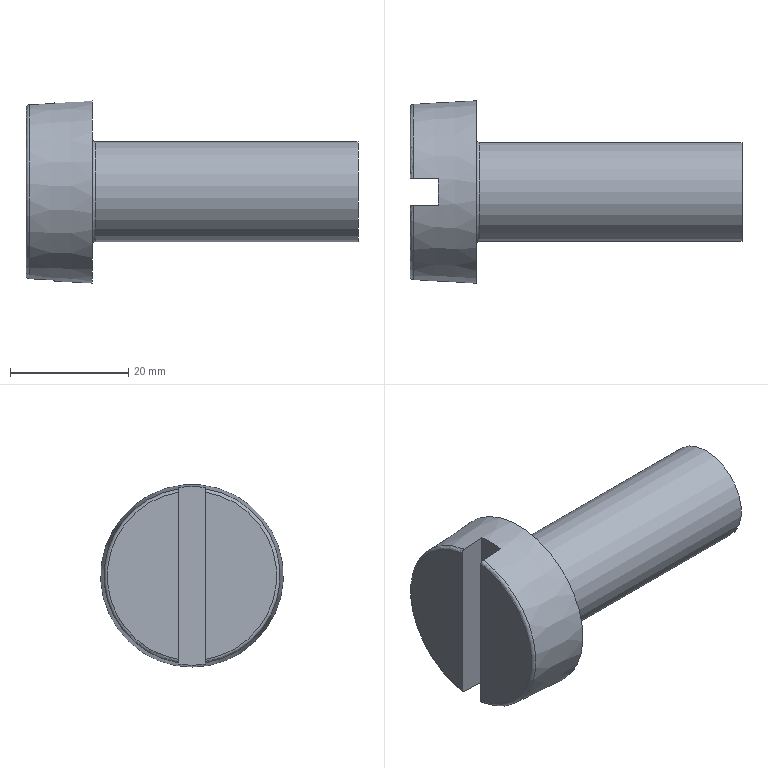Part | NX | features 7.SLDPRT 2, Delete Body 1, LINKED_BODY 1, MOVE_FACE 1, SCALE 1 | 1 solid | 12 faces | box 56.25 x 30.938 x 30.938 mm | volume 17558 mm3 | plane 7 | torus 3 | cone 1 | cylinder 1 | commonest cylinder face diameters 16.875 x1
STEP:
#1=CARTESIAN_POINT('',(-480.939,1888.031,-297.995));
#2=VERTEX_POINT('',#1);
#3=CARTESIAN_POINT('',(-480.939,1888.031,-326.331));
#4=VERTEX_POINT('',#3);
#5=CARTESIAN_POINT('',(-480.939,1888.031,-312.163));
#6=DIRECTION('',(0.,0.,-1.));
#7=VECTOR('',#6,1000.);
#8=LINE('',#5,#7);
#9=EDGE_CURVE('',#2,#4,#8,.T.);
#10=ORIENTED_EDGE('',*,*,#9,.T.);
#11=CARTESIAN_POINT('',(-480.939,1890.281,-312.163));
#12=DIRECTION('',(1.,0.,0.));
#13=DIRECTION('',(0.,0.,-1.));
#14=AXIS2_PLACEMENT_3D('',#11,#12,#13);
#15=CIRCLE('',#14,14.345);
#16=EDGE_CURVE('',#4,#2,#15,.F.);
#17=ORIENTED_EDGE('',*,*,#16,.T.);
#18=EDGE_LOOP('',(#10,#17));
#19=FACE_BOUND('',#18,.T.);
#20=CARTESIAN_POINT('',(-480.939,1890.281,-312.163));
#21=DIRECTION('',(1.,0.,0.));
#22=DIRECTION('',(0.,0.,-1.));
#23=AXIS2_PLACEMENT_3D('',#20,#21,#22);
#24=PLANE('',#23);
#25=ADVANCED_FACE('',(#19),#24,.F.);
#26=CARTESIAN_POINT('',(-469.689,1890.281,-321.163));
#27=VERTEX_POINT('',#26);
#28=CARTESIAN_POINT('',(-469.689,1890.281,-312.163));
#29=DIRECTION('',(1.,0.,0.));
#30=DIRECTION('',(0.,0.,-1.));
#31=AXIS2_PLACEMENT_3D('',#28,#29,#30);
#32=CIRCLE('',#31,9.);
#33=EDGE_CURVE('',#27,#27,#32,.F.);
#34=ORIENTED_EDGE('',*,*,#33,.T.);
#35=EDGE_LOOP('',(#34));
#36=FACE_BOUND('',#35,.T.);
#37=CARTESIAN_POINT('',(-469.689,1890.281,-327.632));
#38=VERTEX_POINT('',#37);
#39=CARTESIAN_POINT('',(-469.689,1890.281,-312.163));
#40=DIRECTION('',(1.,0.,0.));
#41=DIRECTION('',(0.,0.,-1.));
#42=AXIS2_PLACEMENT_3D('',#39,#40,#41);
#43=CIRCLE('',#42,15.469);
#44=EDGE_CURVE('',#38,#38,#43,.T.);
#45=ORIENTED_EDGE('',*,*,#44,.T.);
#46=EDGE_LOOP('',(#45));
#47=FACE_BOUND('',#46,.T.);
#48=CARTESIAN_POINT('',(-469.689,1890.281,-312.163));
#49=DIRECTION('',(1.,0.,0.));
#50=DIRECTION('',(0.,0.,-1.));
#51=AXIS2_PLACEMENT_3D('',#48,#49,#50);
#52=PLANE('',#51);
#53=ADVANCED_FACE('',(#36,#47),#52,.T.);
#54=CARTESIAN_POINT('',(-480.406,1888.031,-297.427));
#55=VERTEX_POINT('',#54);
#56=CARTESIAN_POINT('',(-476.158,1888.031,-297.201));
#57=VERTEX_POINT('',#56);
#58=CARTESIAN_POINT('',(-480.406,1888.031,-297.427));
#59=CARTESIAN_POINT('',(-478.99,1888.031,-297.352));
#60=CARTESIAN_POINT('',(-477.574,1888.031,-297.276));
#61=CARTESIAN_POINT('',(-476.158,1888.031,-297.201));
#62=B_SPLINE_CURVE_WITH_KNOTS('',3,(#58,#59,#60,#61),.UNSPECIFIED.,.F.,.F.,(4,4),(0.02681,0.03107),.UNSPECIFIED.);
#63=EDGE_CURVE('',#55,#57,#62,.T.);
#64=ORIENTED_EDGE('',*,*,#63,.F.);
#65=CARTESIAN_POINT('',(-480.406,1888.031,-326.899));
#66=VERTEX_POINT('',#65);
#67=CARTESIAN_POINT('',(-480.406,1890.281,-312.163));
#68=DIRECTION('',(1.,0.,0.));
#69=DIRECTION('',(0.,0.,-1.));
#70=AXIS2_PLACEMENT_3D('',#67,#68,#69);
#71=CIRCLE('',#70,14.907);
#72=EDGE_CURVE('',#55,#66,#71,.T.);
#73=ORIENTED_EDGE('',*,*,#72,.T.);
#74=CARTESIAN_POINT('',(-476.158,1888.031,-327.124));
#75=VERTEX_POINT('',#74);
#76=CARTESIAN_POINT('',(-476.158,1888.031,-327.124));
#77=CARTESIAN_POINT('',(-477.574,1888.031,-327.049));
#78=CARTESIAN_POINT('',(-478.99,1888.031,-326.974));
#79=CARTESIAN_POINT('',(-480.406,1888.031,-326.899));
#80=B_SPLINE_CURVE_WITH_KNOTS('',3,(#76,#77,#78,#79),.UNSPECIFIED.,.F.,.F.,(4,4),(0.02593,0.03019),.UNSPECIFIED.);
#81=EDGE_CURVE('',#75,#66,#80,.T.);
#82=ORIENTED_EDGE('',*,*,#81,.F.);
#83=CARTESIAN_POINT('',(-476.158,1892.531,-327.124));
#84=VERTEX_POINT('',#83);
#85=CARTESIAN_POINT('',(-476.158,1890.281,-312.163));
#86=DIRECTION('',(1.,0.,0.));
#87=DIRECTION('',(0.,0.,-1.));
#88=AXIS2_PLACEMENT_3D('',#85,#86,#87);
#89=CIRCLE('',#88,15.13);
#90=EDGE_CURVE('',#84,#75,#89,.F.);
#91=ORIENTED_EDGE('',*,*,#90,.F.);
#92=CARTESIAN_POINT('',(-480.406,1892.531,-326.899));
#93=VERTEX_POINT('',#92);
#94=CARTESIAN_POINT('',(-480.406,1892.531,-326.899));
#95=CARTESIAN_POINT('',(-478.99,1892.531,-326.974));
#96=CARTESIAN_POINT('',(-477.574,1892.531,-327.049));
#97=CARTESIAN_POINT('',(-476.158,1892.531,-327.124));
#98=B_SPLINE_CURVE_WITH_KNOTS('',3,(#94,#95,#96,#97),.UNSPECIFIED.,.F.,.F.,(4,4),(0.02681,0.03107),.UNSPECIFIED.);
#99=EDGE_CURVE('',#93,#84,#98,.T.);
#100=ORIENTED_EDGE('',*,*,#99,.F.);
#101=CARTESIAN_POINT('',(-480.406,1892.531,-297.427));
#102=VERTEX_POINT('',#101);
#103=CARTESIAN_POINT('',(-480.406,1890.281,-312.163));
#104=DIRECTION('',(1.,0.,0.));
#105=DIRECTION('',(0.,0.,-1.));
#106=AXIS2_PLACEMENT_3D('',#103,#104,#105);
#107=CIRCLE('',#106,14.907);
#108=EDGE_CURVE('',#93,#102,#107,.T.);
#109=ORIENTED_EDGE('',*,*,#108,.T.);
#110=CARTESIAN_POINT('',(-476.158,1892.531,-297.201));
#111=VERTEX_POINT('',#110);
#112=CARTESIAN_POINT('',(-476.158,1892.531,-297.201));
#113=CARTESIAN_POINT('',(-477.574,1892.531,-297.276));
#114=CARTESIAN_POINT('',(-478.99,1892.531,-297.352));
#115=CARTESIAN_POINT('',(-480.406,1892.531,-297.427));
#116=B_SPLINE_CURVE_WITH_KNOTS('',3,(#112,#113,#114,#115),.UNSPECIFIED.,.F.,.F.,(4,4),(0.02593,0.03019),.UNSPECIFIED.);
#117=EDGE_CURVE('',#111,#102,#116,.T.);
#118=ORIENTED_EDGE('',*,*,#117,.F.);
#119=CARTESIAN_POINT('',(-476.158,1890.281,-312.163));
#120=DIRECTION('',(1.,0.,0.));
#121=DIRECTION('',(0.,0.,-1.));
#122=AXIS2_PLACEMENT_3D('',#119,#120,#121);
#123=CIRCLE('',#122,15.13);
#124=EDGE_CURVE('',#57,#111,#123,.F.);
#125=ORIENTED_EDGE('',*,*,#124,.F.);
#126=EDGE_LOOP('',(#64,#73,#82,#91,#100,#109,#118,#125));
#127=FACE_BOUND('',#126,.T.);
#128=ORIENTED_EDGE('',*,*,#44,.F.);
#129=EDGE_LOOP('',(#128));
#130=FACE_BOUND('',#129,.T.);
#131=CARTESIAN_POINT('',(-469.689,1890.281,-312.163));
#132=DIRECTION('',(1.,0.,0.));
#133=DIRECTION('',(0.,0.,-1.));
#134=AXIS2_PLACEMENT_3D('',#131,#132,#133);
#135=CONICAL_SURFACE('',#134,15.469,0.05236);
#136=ADVANCED_FACE('',(#127,#130),#135,.T.);
#137=CARTESIAN_POINT('',(-480.939,1892.531,-326.331));
#138=VERTEX_POINT('',#137);
#139=CARTESIAN_POINT('',(-480.939,1892.531,-297.995));
#140=VERTEX_POINT('',#139);
#141=CARTESIAN_POINT('',(-480.939,1892.531,-312.163));
#142=DIRECTION('',(0.,0.,1.));
#143=VECTOR('',#142,1000.);
#144=LINE('',#141,#143);
#145=EDGE_CURVE('',#138,#140,#144,.T.);
#146=ORIENTED_EDGE('',*,*,#145,.T.);
#147=CARTESIAN_POINT('',(-480.939,1890.281,-312.163));
#148=DIRECTION('',(1.,0.,0.));
#149=DIRECTION('',(0.,0.,-1.));
#150=AXIS2_PLACEMENT_3D('',#147,#148,#149);
#151=CIRCLE('',#150,14.345);
#152=EDGE_CURVE('',#140,#138,#151,.F.);
#153=ORIENTED_EDGE('',*,*,#152,.T.);
#154=EDGE_LOOP('',(#146,#153));
#155=FACE_BOUND('',#154,.T.);
#156=CARTESIAN_POINT('',(-480.939,1890.281,-312.163));
#157=DIRECTION('',(1.,0.,0.));
#158=DIRECTION('',(0.,0.,-1.));
#159=AXIS2_PLACEMENT_3D('',#156,#157,#158);
#160=PLANE('',#159);
#161=ADVANCED_FACE('',(#155),#160,.F.);
#162=CARTESIAN_POINT('',(-469.126,1890.281,-320.6));
#163=VERTEX_POINT('',#162);
#164=CARTESIAN_POINT('',(-469.126,1890.281,-312.163));
#165=DIRECTION('',(1.,0.,0.));
#166=DIRECTION('',(0.,0.,-1.));
#167=AXIS2_PLACEMENT_3D('',#164,#165,#166);
#168=CIRCLE('',#167,8.438);
#169=EDGE_CURVE('',#163,#163,#168,.T.);
#170=ORIENTED_EDGE('',*,*,#169,.T.);
#171=EDGE_LOOP('',(#170));
#172=FACE_BOUND('',#171,.T.);
#173=CARTESIAN_POINT('',(-424.689,1890.281,-320.6));
#174=VERTEX_POINT('',#173);
#175=CARTESIAN_POINT('',(-424.689,1890.281,-312.163));
#176=DIRECTION('',(1.,0.,0.));
#177=DIRECTION('',(0.,0.,-1.));
#178=AXIS2_PLACEMENT_3D('',#175,#176,#177);
#179=CIRCLE('',#178,8.438);
#180=EDGE_CURVE('',#174,#174,#179,.T.);
#181=ORIENTED_EDGE('',*,*,#180,.F.);
#182=EDGE_LOOP('',(#181));
#183=FACE_BOUND('',#182,.T.);
#184=CARTESIAN_POINT('',(-413.439,1890.281,-312.163));
#185=DIRECTION('',(-1.,0.,0.));
#186=DIRECTION('',(0.,0.,1.));
#187=AXIS2_PLACEMENT_3D('',#184,#185,#186);
#188=CYLINDRICAL_SURFACE('',#187,8.438);
#189=ADVANCED_FACE('',(#172,#183),#188,.T.);
#190=ORIENTED_EDGE('',*,*,#180,.T.);
#191=EDGE_LOOP('',(#190));
#192=FACE_BOUND('',#191,.T.);
#193=CARTESIAN_POINT('',(-424.689,1890.281,-312.163));
#194=DIRECTION('',(1.,0.,0.));
#195=DIRECTION('',(0.,0.,-1.));
#196=AXIS2_PLACEMENT_3D('',#193,#194,#195);
#197=PLANE('',#196);
#198=ADVANCED_FACE('',(#192),#197,.T.);
#199=ORIENTED_EDGE('',*,*,#81,.T.);
#200=CARTESIAN_POINT('',(-480.406,1888.031,-326.899));
#201=CARTESIAN_POINT('',(-480.694,1888.031,-326.884));
#202=CARTESIAN_POINT('',(-480.939,1888.031,-326.62));
#203=CARTESIAN_POINT('',(-480.939,1888.031,-326.331));
#204=B_SPLINE_CURVE_WITH_KNOTS('',3,(#200,#201,#202,#203),.UNSPECIFIED.,.F.,.F.,(4,4),(0.,0.0008547),.UNSPECIFIED.);
#205=EDGE_CURVE('',#66,#4,#204,.T.);
#206=ORIENTED_EDGE('',*,*,#205,.T.);
#207=ORIENTED_EDGE('',*,*,#9,.F.);
#208=CARTESIAN_POINT('',(-480.939,1888.031,-297.995));
#209=CARTESIAN_POINT('',(-480.939,1888.031,-297.706));
#210=CARTESIAN_POINT('',(-480.695,1888.031,-297.442));
#211=CARTESIAN_POINT('',(-480.406,1888.031,-297.427));
#212=B_SPLINE_CURVE_WITH_KNOTS('',3,(#208,#209,#210,#211),.UNSPECIFIED.,.F.,.F.,(4,4),(0.,0.0008548),.UNSPECIFIED.);
#213=EDGE_CURVE('',#2,#55,#212,.T.);
#214=ORIENTED_EDGE('',*,*,#213,.T.);
#215=ORIENTED_EDGE('',*,*,#63,.T.);
#216=CARTESIAN_POINT('',(-476.158,1888.031,-327.632));
#217=DIRECTION('',(0.,0.,1.));
#218=VECTOR('',#217,1000.);
#219=LINE('',#216,#218);
#220=EDGE_CURVE('',#75,#57,#219,.T.);
#221=ORIENTED_EDGE('',*,*,#220,.F.);
#222=EDGE_LOOP('',(#199,#206,#207,#214,#215,#221));
#223=FACE_BOUND('',#222,.T.);
#224=CARTESIAN_POINT('',(-480.939,1888.031,-327.632));
#225=DIRECTION('',(0.,-1.,0.));
#226=DIRECTION('',(1.,0.,0.));
#227=AXIS2_PLACEMENT_3D('',#224,#225,#226);
#228=PLANE('',#227);
#229=ADVANCED_FACE('',(#223),#228,.F.);
#230=ORIENTED_EDGE('',*,*,#117,.T.);
#231=CARTESIAN_POINT('',(-480.406,1892.531,-297.427));
#232=CARTESIAN_POINT('',(-480.694,1892.531,-297.442));
#233=CARTESIAN_POINT('',(-480.939,1892.531,-297.706));
#234=CARTESIAN_POINT('',(-480.939,1892.531,-297.995));
#235=B_SPLINE_CURVE_WITH_KNOTS('',3,(#231,#232,#233,#234),.UNSPECIFIED.,.F.,.F.,(4,4),(0.,0.0008547),.UNSPECIFIED.);
#236=EDGE_CURVE('',#102,#140,#235,.T.);
#237=ORIENTED_EDGE('',*,*,#236,.T.);
#238=ORIENTED_EDGE('',*,*,#145,.F.);
#239=CARTESIAN_POINT('',(-480.939,1892.531,-326.331));
#240=CARTESIAN_POINT('',(-480.939,1892.531,-326.62));
#241=CARTESIAN_POINT('',(-480.695,1892.531,-326.884));
#242=CARTESIAN_POINT('',(-480.406,1892.531,-326.899));
#243=B_SPLINE_CURVE_WITH_KNOTS('',3,(#239,#240,#241,#242),.UNSPECIFIED.,.F.,.F.,(4,4),(0.,0.0008548),.UNSPECIFIED.);
#244=EDGE_CURVE('',#138,#93,#243,.T.);
#245=ORIENTED_EDGE('',*,*,#244,.T.);
#246=ORIENTED_EDGE('',*,*,#99,.T.);
#247=CARTESIAN_POINT('',(-476.158,1892.531,-327.632));
#248=DIRECTION('',(0.,0.,1.));
#249=VECTOR('',#248,1000.);
#250=LINE('',#247,#249);
#251=EDGE_CURVE('',#84,#111,#250,.T.);
#252=ORIENTED_EDGE('',*,*,#251,.T.);
#253=EDGE_LOOP('',(#230,#237,#238,#245,#246,#252));
#254=FACE_BOUND('',#253,.T.);
#255=CARTESIAN_POINT('',(-480.939,1892.531,-327.632));
#256=DIRECTION('',(0.,1.,0.));
#257=DIRECTION('',(0.,0.,1.));
#258=AXIS2_PLACEMENT_3D('',#255,#256,#257);
#259=PLANE('',#258);
#260=ADVANCED_FACE('',(#254),#259,.F.);
#261=ORIENTED_EDGE('',*,*,#124,.T.);
#262=ORIENTED_EDGE('',*,*,#251,.F.);
#263=ORIENTED_EDGE('',*,*,#90,.T.);
#264=ORIENTED_EDGE('',*,*,#220,.T.);
#265=EDGE_LOOP('',(#261,#262,#263,#264));
#266=FACE_BOUND('',#265,.T.);
#267=CARTESIAN_POINT('',(-476.158,1888.031,-327.632));
#268=DIRECTION('',(1.,0.,0.));
#269=DIRECTION('',(0.,0.,-1.));
#270=AXIS2_PLACEMENT_3D('',#267,#268,#269);
#271=PLANE('',#270);
#272=ADVANCED_FACE('',(#266),#271,.F.);
#273=ORIENTED_EDGE('',*,*,#33,.F.);
#274=EDGE_LOOP('',(#273));
#275=FACE_BOUND('',#274,.T.);
#276=ORIENTED_EDGE('',*,*,#169,.F.);
#277=EDGE_LOOP('',(#276));
#278=FACE_BOUND('',#277,.T.);
#279=CARTESIAN_POINT('',(-469.126,1890.281,-312.163));
#280=DIRECTION('',(1.,0.,0.));
#281=DIRECTION('',(0.,0.,-1.));
#282=AXIS2_PLACEMENT_3D('',#279,#280,#281);
#283=TOROIDAL_SURFACE('',#282,9.,0.5625);
#284=ADVANCED_FACE('',(#275,#278),#283,.F.);
#285=ORIENTED_EDGE('',*,*,#213,.F.);
#286=ORIENTED_EDGE('',*,*,#16,.F.);
#287=ORIENTED_EDGE('',*,*,#205,.F.);
#288=ORIENTED_EDGE('',*,*,#72,.F.);
#289=EDGE_LOOP('',(#285,#286,#287,#288));
#290=FACE_BOUND('',#289,.T.);
#291=CARTESIAN_POINT('',(-480.376,1890.281,-312.163));
#292=DIRECTION('',(1.,0.,0.));
#293=DIRECTION('',(0.,0.,-1.));
#294=AXIS2_PLACEMENT_3D('',#291,#292,#293);
#295=TOROIDAL_SURFACE('',#294,14.345,0.5625);
#296=ADVANCED_FACE('',(#290),#295,.T.);
#297=ORIENTED_EDGE('',*,*,#244,.F.);
#298=ORIENTED_EDGE('',*,*,#152,.F.);
#299=ORIENTED_EDGE('',*,*,#236,.F.);
#300=ORIENTED_EDGE('',*,*,#108,.F.);
#301=EDGE_LOOP('',(#297,#298,#299,#300));
#302=FACE_BOUND('',#301,.T.);
#303=CARTESIAN_POINT('',(-480.376,1890.281,-312.163));
#304=DIRECTION('',(1.,0.,0.));
#305=DIRECTION('',(0.,0.,-1.));
#306=AXIS2_PLACEMENT_3D('',#303,#304,#305);
#307=TOROIDAL_SURFACE('',#306,14.345,0.5625);
#308=ADVANCED_FACE('',(#302),#307,.T.);
#309=CLOSED_SHELL('',(#25,#53,#136,#161,#189,#198,#229,#260,#272,#284,#296,#308));
#310=MANIFOLD_SOLID_BREP('',#309);
#311=(LENGTH_UNIT()NAMED_UNIT(*)SI_UNIT(.MILLI.,.METRE.));
#312=UNCERTAINTY_MEASURE_WITH_UNIT(LENGTH_MEASURE(0.0508),#311,'','');
#313=(NAMED_UNIT(*)PLANE_ANGLE_UNIT()SI_UNIT($,.RADIAN.));
#314=(NAMED_UNIT(*)SI_UNIT($,.STERADIAN.)SOLID_ANGLE_UNIT());
#315=(GEOMETRIC_REPRESENTATION_CONTEXT(3)GLOBAL_UNCERTAINTY_ASSIGNED_CONTEXT((#312))GLOBAL_UNIT_ASSIGNED_CONTEXT((#311,#313,#314))REPRESENTATION_CONTEXT('',''));
#316=ADVANCED_BREP_SHAPE_REPRESENTATION('',(#310),#315);